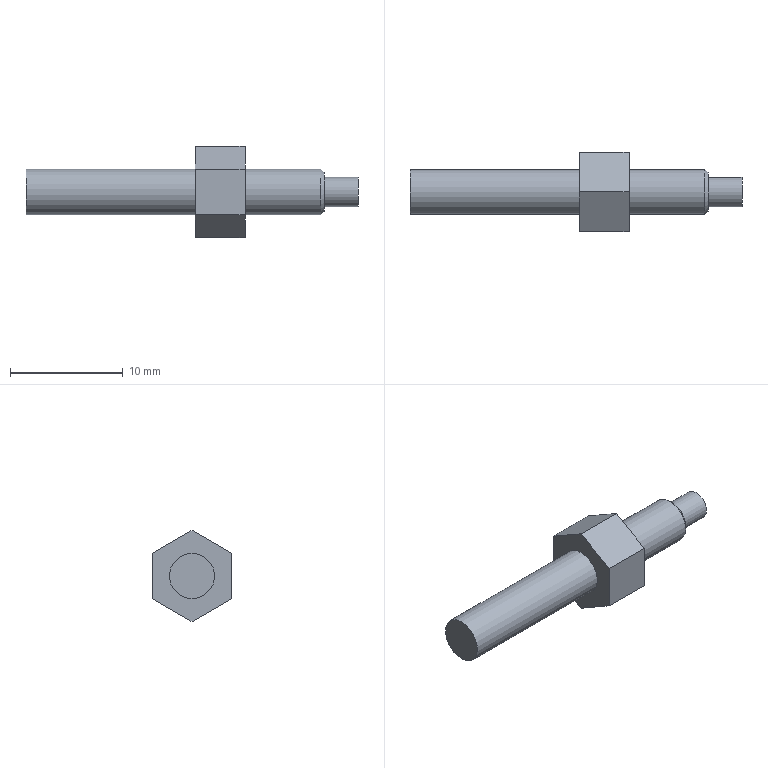Part | NX | 1 solid | 15 faces | box 29.4 x 7 x 8.083 mm | volume 478.566 mm3 | plane 11 | cylinder 3 | cone 1 | commonest cylinder face diameters 4 x2 2.6 x1
STEP:
#1=CARTESIAN_POINT('',(-192.075,-591.6,-44.));
#2=VERTEX_POINT('',#1);
#3=CARTESIAN_POINT('',(-192.075,-591.6,-42.));
#4=DIRECTION('',(1.,0.,0.));
#5=DIRECTION('',(0.,0.,-1.));
#6=AXIS2_PLACEMENT_3D('',#3,#4,#5);
#7=CIRCLE('',#6,2.);
#8=EDGE_CURVE('',#2,#2,#7,.F.);
#9=ORIENTED_EDGE('',*,*,#8,.T.);
#10=EDGE_LOOP('',(#9));
#11=FACE_BOUND('',#10,.T.);
#12=CARTESIAN_POINT('',(-198.775,-591.6,-40.));
#13=VERTEX_POINT('',#12);
#14=CARTESIAN_POINT('',(-198.775,-591.6,-42.));
#15=DIRECTION('',(-1.,0.,0.));
#16=DIRECTION('',(0.,0.,1.));
#17=AXIS2_PLACEMENT_3D('',#14,#15,#16);
#18=CIRCLE('',#17,2.);
#19=EDGE_CURVE('',#13,#13,#18,.T.);
#20=ORIENTED_EDGE('',*,*,#19,.F.);
#21=EDGE_LOOP('',(#20));
#22=FACE_BOUND('',#21,.T.);
#23=CARTESIAN_POINT('',(-191.775,-591.6,-42.));
#24=DIRECTION('',(-1.,0.,0.));
#25=DIRECTION('',(0.,0.,1.));
#26=AXIS2_PLACEMENT_3D('',#23,#24,#25);
#27=CYLINDRICAL_SURFACE('',#26,2.);
#28=ADVANCED_FACE('',(#11,#22),#27,.T.);
#29=CARTESIAN_POINT('',(-191.775,-591.6,-43.7));
#30=VERTEX_POINT('',#29);
#31=CARTESIAN_POINT('',(-191.775,-591.6,-42.));
#32=DIRECTION('',(1.,0.,0.));
#33=DIRECTION('',(0.,0.,-1.));
#34=AXIS2_PLACEMENT_3D('',#31,#32,#33);
#35=CIRCLE('',#34,1.7);
#36=EDGE_CURVE('',#30,#30,#35,.T.);
#37=ORIENTED_EDGE('',*,*,#36,.T.);
#38=EDGE_LOOP('',(#37));
#39=FACE_BOUND('',#38,.T.);
#40=CARTESIAN_POINT('',(-191.775,-591.6,-43.3));
#41=VERTEX_POINT('',#40);
#42=CARTESIAN_POINT('',(-191.775,-591.6,-42.));
#43=DIRECTION('',(1.,0.,0.));
#44=DIRECTION('',(0.,0.,-1.));
#45=AXIS2_PLACEMENT_3D('',#42,#43,#44);
#46=CIRCLE('',#45,1.3);
#47=EDGE_CURVE('',#41,#41,#46,.T.);
#48=ORIENTED_EDGE('',*,*,#47,.F.);
#49=EDGE_LOOP('',(#48));
#50=FACE_BOUND('',#49,.T.);
#51=CARTESIAN_POINT('',(-191.775,-591.6,-42.));
#52=DIRECTION('',(1.,0.,0.));
#53=DIRECTION('',(0.,0.,-1.));
#54=AXIS2_PLACEMENT_3D('',#51,#52,#53);
#55=PLANE('',#54);
#56=ADVANCED_FACE('',(#39,#50),#55,.T.);
#57=CARTESIAN_POINT('',(-188.775,-591.6,-43.3));
#58=VERTEX_POINT('',#57);
#59=CARTESIAN_POINT('',(-188.775,-591.6,-42.));
#60=DIRECTION('',(1.,0.,0.));
#61=DIRECTION('',(0.,0.,-1.));
#62=AXIS2_PLACEMENT_3D('',#59,#60,#61);
#63=CIRCLE('',#62,1.3);
#64=EDGE_CURVE('',#58,#58,#63,.T.);
#65=ORIENTED_EDGE('',*,*,#64,.F.);
#66=EDGE_LOOP('',(#65));
#67=FACE_BOUND('',#66,.T.);
#68=ORIENTED_EDGE('',*,*,#47,.T.);
#69=EDGE_LOOP('',(#68));
#70=FACE_BOUND('',#69,.T.);
#71=CARTESIAN_POINT('',(-188.775,-591.6,-42.));
#72=DIRECTION('',(-1.,0.,0.));
#73=DIRECTION('',(0.,0.,1.));
#74=AXIS2_PLACEMENT_3D('',#71,#72,#73);
#75=CYLINDRICAL_SURFACE('',#74,1.3);
#76=ADVANCED_FACE('',(#67,#70),#75,.T.);
#77=ORIENTED_EDGE('',*,*,#64,.T.);
#78=EDGE_LOOP('',(#77));
#79=FACE_BOUND('',#78,.T.);
#80=CARTESIAN_POINT('',(-188.775,-591.6,-42.));
#81=DIRECTION('',(1.,0.,0.));
#82=DIRECTION('',(0.,0.,-1.));
#83=AXIS2_PLACEMENT_3D('',#80,#81,#82);
#84=PLANE('',#83);
#85=ADVANCED_FACE('',(#79),#84,.T.);
#86=CARTESIAN_POINT('',(-198.775,-595.1,-39.979));
#87=VERTEX_POINT('',#86);
#88=CARTESIAN_POINT('',(-198.775,-591.6,-37.959));
#89=VERTEX_POINT('',#88);
#90=CARTESIAN_POINT('',(-198.775,-595.1,-39.979));
#91=DIRECTION('',(0.,0.866,0.5));
#92=VECTOR('',#91,1000.);
#93=LINE('',#90,#92);
#94=EDGE_CURVE('',#87,#89,#93,.T.);
#95=ORIENTED_EDGE('',*,*,#94,.F.);
#96=CARTESIAN_POINT('',(-198.775,-595.1,-44.021));
#97=VERTEX_POINT('',#96);
#98=CARTESIAN_POINT('',(-198.775,-595.1,-44.021));
#99=DIRECTION('',(0.,0.,1.));
#100=VECTOR('',#99,1000.);
#101=LINE('',#98,#100);
#102=EDGE_CURVE('',#97,#87,#101,.T.);
#103=ORIENTED_EDGE('',*,*,#102,.F.);
#104=CARTESIAN_POINT('',(-198.775,-591.6,-46.041));
#105=VERTEX_POINT('',#104);
#106=CARTESIAN_POINT('',(-198.775,-591.6,-46.041));
#107=DIRECTION('',(0.,-0.866,0.5));
#108=VECTOR('',#107,1000.);
#109=LINE('',#106,#108);
#110=EDGE_CURVE('',#105,#97,#109,.T.);
#111=ORIENTED_EDGE('',*,*,#110,.F.);
#112=CARTESIAN_POINT('',(-198.775,-588.1,-44.021));
#113=VERTEX_POINT('',#112);
#114=CARTESIAN_POINT('',(-198.775,-588.1,-44.021));
#115=DIRECTION('',(0.,-0.866,-0.5));
#116=VECTOR('',#115,1000.);
#117=LINE('',#114,#116);
#118=EDGE_CURVE('',#113,#105,#117,.T.);
#119=ORIENTED_EDGE('',*,*,#118,.F.);
#120=CARTESIAN_POINT('',(-198.775,-588.1,-39.979));
#121=VERTEX_POINT('',#120);
#122=CARTESIAN_POINT('',(-198.775,-588.1,-39.979));
#123=DIRECTION('',(0.,0.,-1.));
#124=VECTOR('',#123,1000.);
#125=LINE('',#122,#124);
#126=EDGE_CURVE('',#121,#113,#125,.T.);
#127=ORIENTED_EDGE('',*,*,#126,.F.);
#128=CARTESIAN_POINT('',(-198.775,-591.6,-37.959));
#129=DIRECTION('',(0.,0.866,-0.5));
#130=VECTOR('',#129,1000.);
#131=LINE('',#128,#130);
#132=EDGE_CURVE('',#89,#121,#131,.T.);
#133=ORIENTED_EDGE('',*,*,#132,.F.);
#134=EDGE_LOOP('',(#95,#103,#111,#119,#127,#133));
#135=FACE_BOUND('',#134,.T.);
#136=ORIENTED_EDGE('',*,*,#19,.T.);
#137=EDGE_LOOP('',(#136));
#138=FACE_BOUND('',#137,.T.);
#139=CARTESIAN_POINT('',(-198.775,-591.6,-42.));
#140=DIRECTION('',(-1.,0.,0.));
#141=DIRECTION('',(0.,0.,1.));
#142=AXIS2_PLACEMENT_3D('',#139,#140,#141);
#143=PLANE('',#142);
#144=ADVANCED_FACE('',(#135,#138),#143,.F.);
#145=CARTESIAN_POINT('',(-203.175,-595.1,-39.979));
#146=VERTEX_POINT('',#145);
#147=CARTESIAN_POINT('',(-203.175,-591.6,-37.959));
#148=VERTEX_POINT('',#147);
#149=CARTESIAN_POINT('',(-203.175,-595.1,-39.979));
#150=DIRECTION('',(0.,0.866,0.5));
#151=VECTOR('',#150,1000.);
#152=LINE('',#149,#151);
#153=EDGE_CURVE('',#146,#148,#152,.T.);
#154=ORIENTED_EDGE('',*,*,#153,.T.);
#155=CARTESIAN_POINT('',(-203.175,-588.1,-39.979));
#156=VERTEX_POINT('',#155);
#157=CARTESIAN_POINT('',(-203.175,-591.6,-37.959));
#158=DIRECTION('',(0.,0.866,-0.5));
#159=VECTOR('',#158,1000.);
#160=LINE('',#157,#159);
#161=EDGE_CURVE('',#148,#156,#160,.T.);
#162=ORIENTED_EDGE('',*,*,#161,.T.);
#163=CARTESIAN_POINT('',(-203.175,-588.1,-44.021));
#164=VERTEX_POINT('',#163);
#165=CARTESIAN_POINT('',(-203.175,-588.1,-39.979));
#166=DIRECTION('',(0.,0.,-1.));
#167=VECTOR('',#166,1000.);
#168=LINE('',#165,#167);
#169=EDGE_CURVE('',#156,#164,#168,.T.);
#170=ORIENTED_EDGE('',*,*,#169,.T.);
#171=CARTESIAN_POINT('',(-203.175,-591.6,-46.041));
#172=VERTEX_POINT('',#171);
#173=CARTESIAN_POINT('',(-203.175,-588.1,-44.021));
#174=DIRECTION('',(0.,-0.866,-0.5));
#175=VECTOR('',#174,1000.);
#176=LINE('',#173,#175);
#177=EDGE_CURVE('',#164,#172,#176,.T.);
#178=ORIENTED_EDGE('',*,*,#177,.T.);
#179=CARTESIAN_POINT('',(-203.175,-595.1,-44.021));
#180=VERTEX_POINT('',#179);
#181=CARTESIAN_POINT('',(-203.175,-591.6,-46.041));
#182=DIRECTION('',(0.,-0.866,0.5));
#183=VECTOR('',#182,1000.);
#184=LINE('',#181,#183);
#185=EDGE_CURVE('',#172,#180,#184,.T.);
#186=ORIENTED_EDGE('',*,*,#185,.T.);
#187=CARTESIAN_POINT('',(-203.175,-595.1,-44.021));
#188=DIRECTION('',(0.,0.,1.));
#189=VECTOR('',#188,1000.);
#190=LINE('',#187,#189);
#191=EDGE_CURVE('',#180,#146,#190,.T.);
#192=ORIENTED_EDGE('',*,*,#191,.T.);
#193=EDGE_LOOP('',(#154,#162,#170,#178,#186,#192));
#194=FACE_BOUND('',#193,.T.);
#195=CARTESIAN_POINT('',(-203.175,-591.6,-40.));
#196=VERTEX_POINT('',#195);
#197=CARTESIAN_POINT('',(-203.175,-591.6,-42.));
#198=DIRECTION('',(-1.,0.,0.));
#199=DIRECTION('',(0.,0.,1.));
#200=AXIS2_PLACEMENT_3D('',#197,#198,#199);
#201=CIRCLE('',#200,2.);
#202=EDGE_CURVE('',#196,#196,#201,.T.);
#203=ORIENTED_EDGE('',*,*,#202,.F.);
#204=EDGE_LOOP('',(#203));
#205=FACE_BOUND('',#204,.T.);
#206=CARTESIAN_POINT('',(-203.175,-591.6,-42.));
#207=DIRECTION('',(-1.,0.,0.));
#208=DIRECTION('',(0.,0.,1.));
#209=AXIS2_PLACEMENT_3D('',#206,#207,#208);
#210=PLANE('',#209);
#211=ADVANCED_FACE('',(#194,#205),#210,.T.);
#212=ORIENTED_EDGE('',*,*,#153,.F.);
#213=CARTESIAN_POINT('',(-198.775,-595.1,-39.979));
#214=DIRECTION('',(-1.,0.,0.));
#215=VECTOR('',#214,1000.);
#216=LINE('',#213,#215);
#217=EDGE_CURVE('',#87,#146,#216,.T.);
#218=ORIENTED_EDGE('',*,*,#217,.F.);
#219=ORIENTED_EDGE('',*,*,#94,.T.);
#220=CARTESIAN_POINT('',(-198.775,-591.6,-37.959));
#221=DIRECTION('',(-1.,0.,0.));
#222=VECTOR('',#221,1000.);
#223=LINE('',#220,#222);
#224=EDGE_CURVE('',#89,#148,#223,.T.);
#225=ORIENTED_EDGE('',*,*,#224,.T.);
#226=EDGE_LOOP('',(#212,#218,#219,#225));
#227=FACE_BOUND('',#226,.T.);
#228=CARTESIAN_POINT('',(-198.775,-595.1,-39.979));
#229=DIRECTION('',(0.,-0.5,0.866));
#230=DIRECTION('',(0.,-0.866,-0.5));
#231=AXIS2_PLACEMENT_3D('',#228,#229,#230);
#232=PLANE('',#231);
#233=ADVANCED_FACE('',(#227),#232,.T.);
#234=ORIENTED_EDGE('',*,*,#191,.F.);
#235=CARTESIAN_POINT('',(-198.775,-595.1,-44.021));
#236=DIRECTION('',(-1.,0.,0.));
#237=VECTOR('',#236,1000.);
#238=LINE('',#235,#237);
#239=EDGE_CURVE('',#97,#180,#238,.T.);
#240=ORIENTED_EDGE('',*,*,#239,.F.);
#241=ORIENTED_EDGE('',*,*,#102,.T.);
#242=ORIENTED_EDGE('',*,*,#217,.T.);
#243=EDGE_LOOP('',(#234,#240,#241,#242));
#244=FACE_BOUND('',#243,.T.);
#245=CARTESIAN_POINT('',(-198.775,-595.1,-44.021));
#246=DIRECTION('',(0.,-1.,0.));
#247=DIRECTION('',(0.,0.,-1.));
#248=AXIS2_PLACEMENT_3D('',#245,#246,#247);
#249=PLANE('',#248);
#250=ADVANCED_FACE('',(#244),#249,.T.);
#251=ORIENTED_EDGE('',*,*,#185,.F.);
#252=CARTESIAN_POINT('',(-198.775,-591.6,-46.041));
#253=DIRECTION('',(-1.,0.,0.));
#254=VECTOR('',#253,1000.);
#255=LINE('',#252,#254);
#256=EDGE_CURVE('',#105,#172,#255,.T.);
#257=ORIENTED_EDGE('',*,*,#256,.F.);
#258=ORIENTED_EDGE('',*,*,#110,.T.);
#259=ORIENTED_EDGE('',*,*,#239,.T.);
#260=EDGE_LOOP('',(#251,#257,#258,#259));
#261=FACE_BOUND('',#260,.T.);
#262=CARTESIAN_POINT('',(-198.775,-591.6,-46.041));
#263=DIRECTION('',(0.,-0.5,-0.866));
#264=DIRECTION('',(0.,0.866,-0.5));
#265=AXIS2_PLACEMENT_3D('',#262,#263,#264);
#266=PLANE('',#265);
#267=ADVANCED_FACE('',(#261),#266,.T.);
#268=ORIENTED_EDGE('',*,*,#177,.F.);
#269=CARTESIAN_POINT('',(-198.775,-588.1,-44.021));
#270=DIRECTION('',(-1.,0.,0.));
#271=VECTOR('',#270,1000.);
#272=LINE('',#269,#271);
#273=EDGE_CURVE('',#113,#164,#272,.T.);
#274=ORIENTED_EDGE('',*,*,#273,.F.);
#275=ORIENTED_EDGE('',*,*,#118,.T.);
#276=ORIENTED_EDGE('',*,*,#256,.T.);
#277=EDGE_LOOP('',(#268,#274,#275,#276));
#278=FACE_BOUND('',#277,.T.);
#279=CARTESIAN_POINT('',(-198.775,-588.1,-44.021));
#280=DIRECTION('',(0.,0.5,-0.866));
#281=DIRECTION('',(0.,0.866,0.5));
#282=AXIS2_PLACEMENT_3D('',#279,#280,#281);
#283=PLANE('',#282);
#284=ADVANCED_FACE('',(#278),#283,.T.);
#285=ORIENTED_EDGE('',*,*,#169,.F.);
#286=CARTESIAN_POINT('',(-198.775,-588.1,-39.979));
#287=DIRECTION('',(-1.,0.,0.));
#288=VECTOR('',#287,1000.);
#289=LINE('',#286,#288);
#290=EDGE_CURVE('',#121,#156,#289,.T.);
#291=ORIENTED_EDGE('',*,*,#290,.F.);
#292=ORIENTED_EDGE('',*,*,#126,.T.);
#293=ORIENTED_EDGE('',*,*,#273,.T.);
#294=EDGE_LOOP('',(#285,#291,#292,#293));
#295=FACE_BOUND('',#294,.T.);
#296=CARTESIAN_POINT('',(-198.775,-588.1,-39.979));
#297=DIRECTION('',(0.,1.,0.));
#298=DIRECTION('',(0.,0.,1.));
#299=AXIS2_PLACEMENT_3D('',#296,#297,#298);
#300=PLANE('',#299);
#301=ADVANCED_FACE('',(#295),#300,.T.);
#302=ORIENTED_EDGE('',*,*,#161,.F.);
#303=ORIENTED_EDGE('',*,*,#224,.F.);
#304=ORIENTED_EDGE('',*,*,#132,.T.);
#305=ORIENTED_EDGE('',*,*,#290,.T.);
#306=EDGE_LOOP('',(#302,#303,#304,#305));
#307=FACE_BOUND('',#306,.T.);
#308=CARTESIAN_POINT('',(-198.775,-591.6,-37.959));
#309=DIRECTION('',(0.,0.5,0.866));
#310=DIRECTION('',(0.,-0.866,0.5));
#311=AXIS2_PLACEMENT_3D('',#308,#309,#310);
#312=PLANE('',#311);
#313=ADVANCED_FACE('',(#307),#312,.T.);
#314=CARTESIAN_POINT('',(-218.175,-591.6,-44.));
#315=VERTEX_POINT('',#314);
#316=CARTESIAN_POINT('',(-218.175,-591.6,-42.));
#317=DIRECTION('',(1.,0.,0.));
#318=DIRECTION('',(0.,0.,-1.));
#319=AXIS2_PLACEMENT_3D('',#316,#317,#318);
#320=CIRCLE('',#319,2.);
#321=EDGE_CURVE('',#315,#315,#320,.T.);
#322=ORIENTED_EDGE('',*,*,#321,.F.);
#323=EDGE_LOOP('',(#322));
#324=FACE_BOUND('',#323,.T.);
#325=CARTESIAN_POINT('',(-218.175,-591.6,-42.));
#326=DIRECTION('',(1.,0.,0.));
#327=DIRECTION('',(0.,0.,-1.));
#328=AXIS2_PLACEMENT_3D('',#325,#326,#327);
#329=PLANE('',#328);
#330=ADVANCED_FACE('',(#324),#329,.F.);
#331=ORIENTED_EDGE('',*,*,#202,.T.);
#332=EDGE_LOOP('',(#331));
#333=FACE_BOUND('',#332,.T.);
#334=ORIENTED_EDGE('',*,*,#321,.T.);
#335=EDGE_LOOP('',(#334));
#336=FACE_BOUND('',#335,.T.);
#337=CARTESIAN_POINT('',(-191.775,-591.6,-42.));
#338=DIRECTION('',(-1.,0.,0.));
#339=DIRECTION('',(0.,0.,1.));
#340=AXIS2_PLACEMENT_3D('',#337,#338,#339);
#341=CYLINDRICAL_SURFACE('',#340,2.);
#342=ADVANCED_FACE('',(#333,#336),#341,.T.);
#343=ORIENTED_EDGE('',*,*,#8,.F.);
#344=EDGE_LOOP('',(#343));
#345=FACE_BOUND('',#344,.T.);
#346=ORIENTED_EDGE('',*,*,#36,.F.);
#347=EDGE_LOOP('',(#346));
#348=FACE_BOUND('',#347,.T.);
#349=CARTESIAN_POINT('',(-191.775,-591.6,-42.));
#350=DIRECTION('',(-1.,0.,0.));
#351=DIRECTION('',(0.,0.,1.));
#352=AXIS2_PLACEMENT_3D('',#349,#350,#351);
#353=CONICAL_SURFACE('',#352,1.7,0.7854);
#354=ADVANCED_FACE('',(#345,#348),#353,.T.);
#355=CLOSED_SHELL('',(#28,#56,#76,#85,#144,#211,#233,#250,#267,#284,#301,#313,#330,#342,#354));
#356=MANIFOLD_SOLID_BREP('',#355);
#357=(LENGTH_UNIT()NAMED_UNIT(*)SI_UNIT(.MILLI.,.METRE.));
#358=UNCERTAINTY_MEASURE_WITH_UNIT(LENGTH_MEASURE(0.00001),#357,'','');
#359=(NAMED_UNIT(*)PLANE_ANGLE_UNIT()SI_UNIT($,.RADIAN.));
#360=(NAMED_UNIT(*)SI_UNIT($,.STERADIAN.)SOLID_ANGLE_UNIT());
#361=(GEOMETRIC_REPRESENTATION_CONTEXT(3)GLOBAL_UNCERTAINTY_ASSIGNED_CONTEXT((#358))GLOBAL_UNIT_ASSIGNED_CONTEXT((#357,#359,#360))REPRESENTATION_CONTEXT('',''));
#362=ADVANCED_BREP_SHAPE_REPRESENTATION('',(#356),#361);